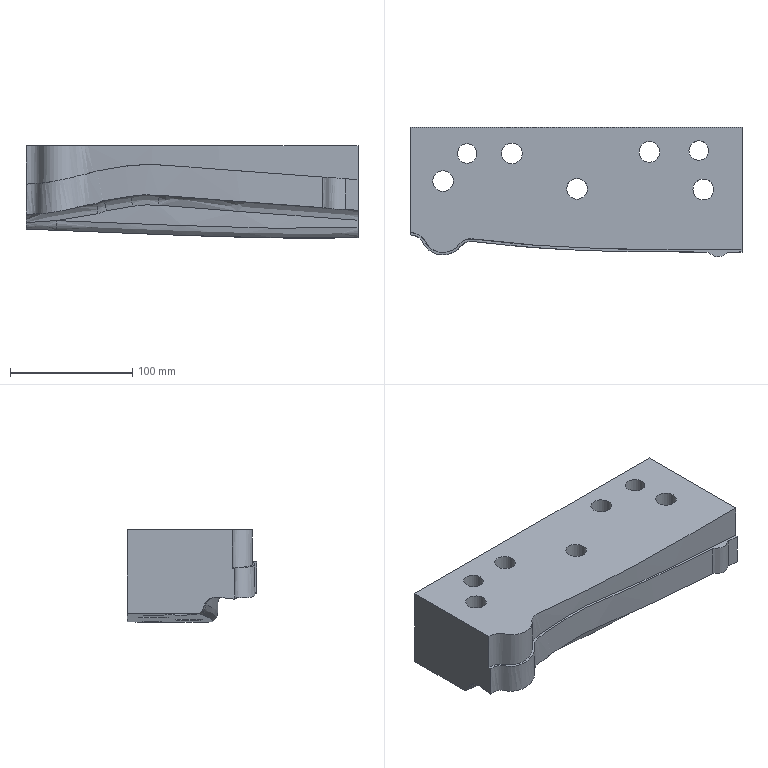Part | NX | features solid 2 | 1 solid | 50 faces | box 271.968 x 106.036 x 75.613 mm | volume 1602157 mm3 | spline 27 | cylinder 14 | plane 9 | commonest cylinder face diameters 17 x7 25 x5 16 x2